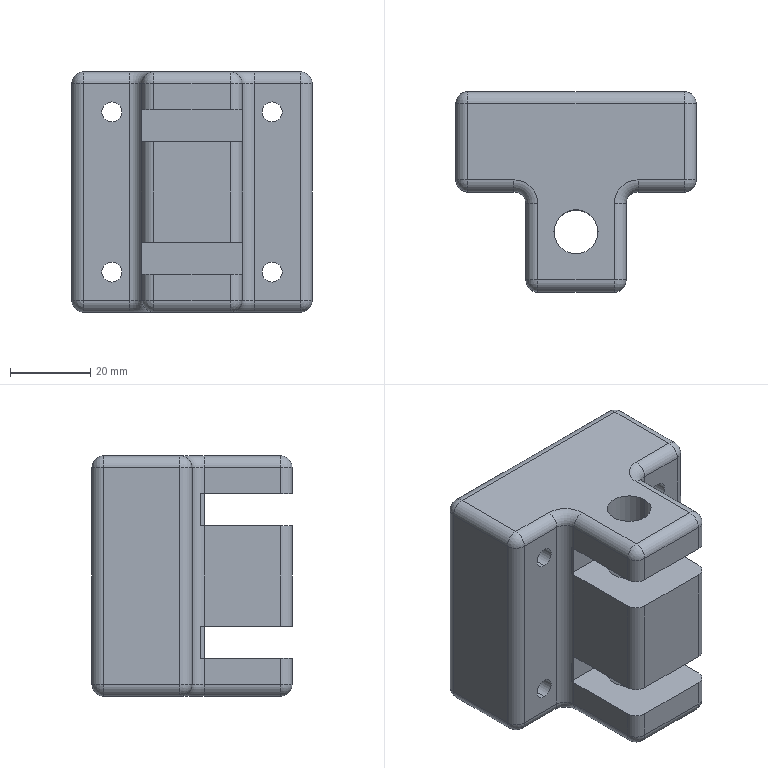Part | SolidWorks | features ICE 2, Extrusion 1, Fillet 1 | 1 solid | 84 faces | box 60 x 50 x 60 mm | volume 110960 mm3 | cylinder 42 | plane 26 | sphere 12 | torus 4 | commonest cylinder face diameters 6 x28 5 x8 11 x6